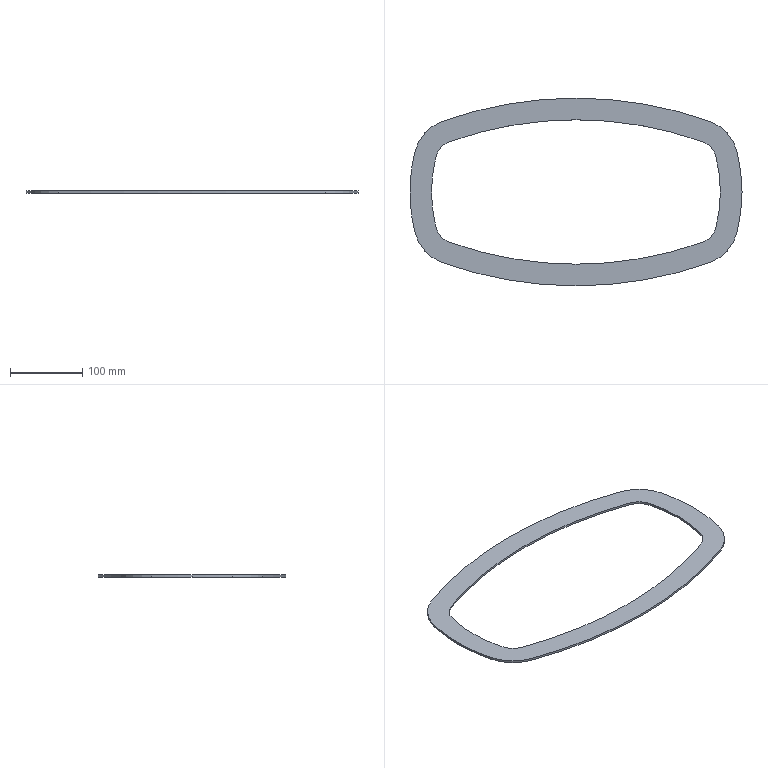Part | SolidWorks | features Extrusion 1 | 1 solid | 20 faces | box 460 x 260 x 3 mm | volume 101049 mm3 | cylinder 18 | plane 2 | commonest cylinder face diameters 60 x4 120 x4 400 x3 460 x3 1040 x2 1100 x2
STEP:
#1=CARTESIAN_POINT('',(-193.97,48.739,3.));
#2=VERTEX_POINT('',#1);
#3=CARTESIAN_POINT('',(-200.,0.,3.));
#4=VERTEX_POINT('',#3);
#5=CARTESIAN_POINT('',(0.,0.,3.));
#6=DIRECTION('',(0.,0.,1.));
#7=DIRECTION('',(-1.,0.,0.));
#8=AXIS2_PLACEMENT_3D('',#5,#6,#7);
#9=CIRCLE('',#8,200.);
#10=EDGE_CURVE('',#2,#4,#9,.T.);
#11=ORIENTED_EDGE('',*,*,#10,.T.);
#12=CARTESIAN_POINT('',(-200.,0.,0.));
#13=VERTEX_POINT('',#12);
#14=CARTESIAN_POINT('',(-200.,0.,3.));
#15=DIRECTION('',(0.,0.,-1.));
#16=VECTOR('',#15,1000.);
#17=LINE('',#14,#16);
#18=EDGE_CURVE('',#4,#13,#17,.T.);
#19=ORIENTED_EDGE('',*,*,#18,.T.);
#20=CARTESIAN_POINT('',(-193.97,48.739,0.));
#21=VERTEX_POINT('',#20);
#22=CARTESIAN_POINT('',(0.,0.,0.));
#23=DIRECTION('',(0.,0.,1.));
#24=DIRECTION('',(-1.,0.,0.));
#25=AXIS2_PLACEMENT_3D('',#22,#23,#24);
#26=CIRCLE('',#25,200.);
#27=EDGE_CURVE('',#21,#13,#26,.T.);
#28=ORIENTED_EDGE('',*,*,#27,.F.);
#29=CARTESIAN_POINT('',(-193.97,48.739,3.));
#30=DIRECTION('',(0.,0.,-1.));
#31=VECTOR('',#30,1000.);
#32=LINE('',#29,#31);
#33=EDGE_CURVE('',#2,#21,#32,.T.);
#34=ORIENTED_EDGE('',*,*,#33,.F.);
#35=EDGE_LOOP('',(#11,#19,#28,#34));
#36=FACE_OUTER_BOUND('',#35,.T.);
#37=CARTESIAN_POINT('',(0.,0.,3.));
#38=DIRECTION('',(0.,0.,-1.));
#39=DIRECTION('',(-1.,0.,0.));
#40=AXIS2_PLACEMENT_3D('',#37,#38,#39);
#41=CYLINDRICAL_SURFACE('',#40,200.);
#42=ADVANCED_FACE('',(#36),#41,.F.);
#43=CARTESIAN_POINT('',(-230.,0.,3.));
#44=VERTEX_POINT('',#43);
#45=CARTESIAN_POINT('',(-223.066,-56.05,3.));
#46=VERTEX_POINT('',#45);
#47=CARTESIAN_POINT('',(0.,0.,3.));
#48=DIRECTION('',(0.,0.,1.));
#49=DIRECTION('',(-1.,0.,0.));
#50=AXIS2_PLACEMENT_3D('',#47,#48,#49);
#51=CIRCLE('',#50,230.);
#52=EDGE_CURVE('',#44,#46,#51,.T.);
#53=ORIENTED_EDGE('',*,*,#52,.F.);
#54=CARTESIAN_POINT('',(-230.,0.,0.));
#55=VERTEX_POINT('',#54);
#56=CARTESIAN_POINT('',(-230.,0.,3.));
#57=DIRECTION('',(0.,0.,-1.));
#58=VECTOR('',#57,1000.);
#59=LINE('',#56,#58);
#60=EDGE_CURVE('',#44,#55,#59,.T.);
#61=ORIENTED_EDGE('',*,*,#60,.T.);
#62=CARTESIAN_POINT('',(-223.066,-56.05,0.));
#63=VERTEX_POINT('',#62);
#64=CARTESIAN_POINT('',(0.,0.,0.));
#65=DIRECTION('',(0.,0.,1.));
#66=DIRECTION('',(-1.,0.,0.));
#67=AXIS2_PLACEMENT_3D('',#64,#65,#66);
#68=CIRCLE('',#67,230.);
#69=EDGE_CURVE('',#55,#63,#68,.T.);
#70=ORIENTED_EDGE('',*,*,#69,.T.);
#71=CARTESIAN_POINT('',(-223.066,-56.05,3.));
#72=DIRECTION('',(0.,0.,-1.));
#73=VECTOR('',#72,1000.);
#74=LINE('',#71,#73);
#75=EDGE_CURVE('',#46,#63,#74,.T.);
#76=ORIENTED_EDGE('',*,*,#75,.F.);
#77=EDGE_LOOP('',(#53,#61,#70,#76));
#78=FACE_OUTER_BOUND('',#77,.T.);
#79=CARTESIAN_POINT('',(0.,0.,3.));
#80=DIRECTION('',(0.,0.,-1.));
#81=DIRECTION('',(-1.,0.,0.));
#82=AXIS2_PLACEMENT_3D('',#79,#80,#81);
#83=CYLINDRICAL_SURFACE('',#82,230.);
#84=ADVANCED_FACE('',(#78),#83,.T.);
#85=CARTESIAN_POINT('',(-185.063,97.93,3.));
#86=VERTEX_POINT('',#85);
#87=CARTESIAN_POINT('',(-223.066,56.05,3.));
#88=VERTEX_POINT('',#87);
#89=CARTESIAN_POINT('',(-164.875,41.429,3.));
#90=DIRECTION('',(0.,0.,1.));
#91=DIRECTION('',(1.,0.,0.));
#92=AXIS2_PLACEMENT_3D('',#89,#90,#91);
#93=CIRCLE('',#92,60.);
#94=EDGE_CURVE('',#86,#88,#93,.T.);
#95=ORIENTED_EDGE('',*,*,#94,.T.);
#96=CARTESIAN_POINT('',(0.,0.,3.));
#97=DIRECTION('',(0.,0.,1.));
#98=DIRECTION('',(-1.,0.,0.));
#99=AXIS2_PLACEMENT_3D('',#96,#97,#98);
#100=CIRCLE('',#99,230.);
#101=EDGE_CURVE('',#88,#44,#100,.T.);
#102=ORIENTED_EDGE('',*,*,#101,.T.);
#103=ORIENTED_EDGE('',*,*,#52,.T.);
#104=CARTESIAN_POINT('',(-185.063,-97.93,3.));
#105=VERTEX_POINT('',#104);
#106=CARTESIAN_POINT('',(-164.875,-41.429,3.));
#107=DIRECTION('',(0.,0.,1.));
#108=DIRECTION('',(-1.,0.,0.));
#109=AXIS2_PLACEMENT_3D('',#106,#107,#108);
#110=CIRCLE('',#109,60.);
#111=EDGE_CURVE('',#46,#105,#110,.T.);
#112=ORIENTED_EDGE('',*,*,#111,.T.);
#113=CARTESIAN_POINT('',(185.063,-97.93,3.));
#114=VERTEX_POINT('',#113);
#115=CARTESIAN_POINT('',(0.,420.,3.));
#116=DIRECTION('',(0.,0.,1.));
#117=DIRECTION('',(1.,0.,0.));
#118=AXIS2_PLACEMENT_3D('',#115,#116,#117);
#119=CIRCLE('',#118,550.);
#120=EDGE_CURVE('',#105,#114,#119,.T.);
#121=ORIENTED_EDGE('',*,*,#120,.T.);
#122=CARTESIAN_POINT('',(223.066,-56.05,3.));
#123=VERTEX_POINT('',#122);
#124=CARTESIAN_POINT('',(164.875,-41.429,3.));
#125=DIRECTION('',(0.,0.,1.));
#126=DIRECTION('',(1.,0.,0.));
#127=AXIS2_PLACEMENT_3D('',#124,#125,#126);
#128=CIRCLE('',#127,60.);
#129=EDGE_CURVE('',#114,#123,#128,.T.);
#130=ORIENTED_EDGE('',*,*,#129,.T.);
#131=CARTESIAN_POINT('',(223.066,56.05,3.));
#132=VERTEX_POINT('',#131);
#133=CARTESIAN_POINT('',(0.,0.,3.));
#134=DIRECTION('',(0.,0.,1.));
#135=DIRECTION('',(-1.,0.,0.));
#136=AXIS2_PLACEMENT_3D('',#133,#134,#135);
#137=CIRCLE('',#136,230.);
#138=EDGE_CURVE('',#123,#132,#137,.T.);
#139=ORIENTED_EDGE('',*,*,#138,.T.);
#140=CARTESIAN_POINT('',(185.063,97.93,3.));
#141=VERTEX_POINT('',#140);
#142=CARTESIAN_POINT('',(164.875,41.429,3.));
#143=DIRECTION('',(0.,0.,1.));
#144=DIRECTION('',(-1.,0.,0.));
#145=AXIS2_PLACEMENT_3D('',#142,#143,#144);
#146=CIRCLE('',#145,60.);
#147=EDGE_CURVE('',#132,#141,#146,.T.);
#148=ORIENTED_EDGE('',*,*,#147,.T.);
#149=CARTESIAN_POINT('',(0.,-420.,3.));
#150=DIRECTION('',(0.,0.,1.));
#151=DIRECTION('',(-1.,0.,0.));
#152=AXIS2_PLACEMENT_3D('',#149,#150,#151);
#153=CIRCLE('',#152,550.);
#154=EDGE_CURVE('',#141,#86,#153,.T.);
#155=ORIENTED_EDGE('',*,*,#154,.T.);
#156=EDGE_LOOP('',(#95,#102,#103,#112,#121,#130,#139,#148,#155));
#157=FACE_OUTER_BOUND('',#156,.T.);
#158=CARTESIAN_POINT('',(193.97,-48.739,3.));
#159=VERTEX_POINT('',#158);
#160=CARTESIAN_POINT('',(193.97,48.739,3.));
#161=VERTEX_POINT('',#160);
#162=CARTESIAN_POINT('',(0.,0.,3.));
#163=DIRECTION('',(0.,0.,1.));
#164=DIRECTION('',(-1.,0.,0.));
#165=AXIS2_PLACEMENT_3D('',#162,#163,#164);
#166=CIRCLE('',#165,200.);
#167=EDGE_CURVE('',#159,#161,#166,.T.);
#168=ORIENTED_EDGE('',*,*,#167,.F.);
#169=CARTESIAN_POINT('',(174.969,-69.679,3.));
#170=VERTEX_POINT('',#169);
#171=CARTESIAN_POINT('',(164.875,-41.429,3.));
#172=DIRECTION('',(0.,0.,1.));
#173=DIRECTION('',(1.,0.,0.));
#174=AXIS2_PLACEMENT_3D('',#171,#172,#173);
#175=CIRCLE('',#174,30.);
#176=EDGE_CURVE('',#170,#159,#175,.T.);
#177=ORIENTED_EDGE('',*,*,#176,.F.);
#178=CARTESIAN_POINT('',(-174.969,-69.679,3.));
#179=VERTEX_POINT('',#178);
#180=CARTESIAN_POINT('',(0.,420.,3.));
#181=DIRECTION('',(0.,0.,1.));
#182=DIRECTION('',(1.,0.,0.));
#183=AXIS2_PLACEMENT_3D('',#180,#181,#182);
#184=CIRCLE('',#183,520.);
#185=EDGE_CURVE('',#179,#170,#184,.T.);
#186=ORIENTED_EDGE('',*,*,#185,.F.);
#187=CARTESIAN_POINT('',(-193.97,-48.739,3.));
#188=VERTEX_POINT('',#187);
#189=CARTESIAN_POINT('',(-164.875,-41.429,3.));
#190=DIRECTION('',(0.,0.,1.));
#191=DIRECTION('',(-1.,0.,0.));
#192=AXIS2_PLACEMENT_3D('',#189,#190,#191);
#193=CIRCLE('',#192,30.);
#194=EDGE_CURVE('',#188,#179,#193,.T.);
#195=ORIENTED_EDGE('',*,*,#194,.F.);
#196=CARTESIAN_POINT('',(0.,0.,3.));
#197=DIRECTION('',(0.,0.,1.));
#198=DIRECTION('',(-1.,0.,0.));
#199=AXIS2_PLACEMENT_3D('',#196,#197,#198);
#200=CIRCLE('',#199,200.);
#201=EDGE_CURVE('',#4,#188,#200,.T.);
#202=ORIENTED_EDGE('',*,*,#201,.F.);
#203=ORIENTED_EDGE('',*,*,#10,.F.);
#204=CARTESIAN_POINT('',(-174.969,69.679,3.));
#205=VERTEX_POINT('',#204);
#206=CARTESIAN_POINT('',(-164.875,41.429,3.));
#207=DIRECTION('',(0.,0.,1.));
#208=DIRECTION('',(1.,0.,0.));
#209=AXIS2_PLACEMENT_3D('',#206,#207,#208);
#210=CIRCLE('',#209,30.);
#211=EDGE_CURVE('',#205,#2,#210,.T.);
#212=ORIENTED_EDGE('',*,*,#211,.F.);
#213=CARTESIAN_POINT('',(174.969,69.679,3.));
#214=VERTEX_POINT('',#213);
#215=CARTESIAN_POINT('',(0.,-420.,3.));
#216=DIRECTION('',(0.,0.,1.));
#217=DIRECTION('',(-1.,0.,0.));
#218=AXIS2_PLACEMENT_3D('',#215,#216,#217);
#219=CIRCLE('',#218,520.);
#220=EDGE_CURVE('',#214,#205,#219,.T.);
#221=ORIENTED_EDGE('',*,*,#220,.F.);
#222=CARTESIAN_POINT('',(164.875,41.429,3.));
#223=DIRECTION('',(0.,0.,1.));
#224=DIRECTION('',(-1.,0.,0.));
#225=AXIS2_PLACEMENT_3D('',#222,#223,#224);
#226=CIRCLE('',#225,30.);
#227=EDGE_CURVE('',#161,#214,#226,.T.);
#228=ORIENTED_EDGE('',*,*,#227,.F.);
#229=EDGE_LOOP('',(#168,#177,#186,#195,#202,#203,#212,#221,#228));
#230=FACE_BOUND('',#229,.T.);
#231=CARTESIAN_POINT('',(-82.437,20.714,3.));
#232=DIRECTION('',(0.,0.,1.));
#233=DIRECTION('',(1.,0.,0.));
#234=AXIS2_PLACEMENT_3D('',#231,#232,#233);
#235=PLANE('',#234);
#236=ADVANCED_FACE('',(#157,#230),#235,.T.);
#237=CARTESIAN_POINT('',(-185.063,97.93,0.));
#238=VERTEX_POINT('',#237);
#239=CARTESIAN_POINT('',(-223.066,56.05,0.));
#240=VERTEX_POINT('',#239);
#241=CARTESIAN_POINT('',(-164.875,41.429,0.));
#242=DIRECTION('',(0.,0.,1.));
#243=DIRECTION('',(1.,0.,0.));
#244=AXIS2_PLACEMENT_3D('',#241,#242,#243);
#245=CIRCLE('',#244,60.);
#246=EDGE_CURVE('',#238,#240,#245,.T.);
#247=ORIENTED_EDGE('',*,*,#246,.F.);
#248=CARTESIAN_POINT('',(185.063,97.93,0.));
#249=VERTEX_POINT('',#248);
#250=CARTESIAN_POINT('',(0.,-420.,0.));
#251=DIRECTION('',(0.,0.,1.));
#252=DIRECTION('',(-1.,0.,0.));
#253=AXIS2_PLACEMENT_3D('',#250,#251,#252);
#254=CIRCLE('',#253,550.);
#255=EDGE_CURVE('',#249,#238,#254,.T.);
#256=ORIENTED_EDGE('',*,*,#255,.F.);
#257=CARTESIAN_POINT('',(223.066,56.05,0.));
#258=VERTEX_POINT('',#257);
#259=CARTESIAN_POINT('',(164.875,41.429,0.));
#260=DIRECTION('',(0.,0.,1.));
#261=DIRECTION('',(-1.,0.,0.));
#262=AXIS2_PLACEMENT_3D('',#259,#260,#261);
#263=CIRCLE('',#262,60.);
#264=EDGE_CURVE('',#258,#249,#263,.T.);
#265=ORIENTED_EDGE('',*,*,#264,.F.);
#266=CARTESIAN_POINT('',(223.066,-56.05,0.));
#267=VERTEX_POINT('',#266);
#268=CARTESIAN_POINT('',(0.,0.,0.));
#269=DIRECTION('',(0.,0.,1.));
#270=DIRECTION('',(-1.,0.,0.));
#271=AXIS2_PLACEMENT_3D('',#268,#269,#270);
#272=CIRCLE('',#271,230.);
#273=EDGE_CURVE('',#267,#258,#272,.T.);
#274=ORIENTED_EDGE('',*,*,#273,.F.);
#275=CARTESIAN_POINT('',(185.063,-97.93,0.));
#276=VERTEX_POINT('',#275);
#277=CARTESIAN_POINT('',(164.875,-41.429,0.));
#278=DIRECTION('',(0.,0.,1.));
#279=DIRECTION('',(1.,0.,0.));
#280=AXIS2_PLACEMENT_3D('',#277,#278,#279);
#281=CIRCLE('',#280,60.);
#282=EDGE_CURVE('',#276,#267,#281,.T.);
#283=ORIENTED_EDGE('',*,*,#282,.F.);
#284=CARTESIAN_POINT('',(-185.063,-97.93,0.));
#285=VERTEX_POINT('',#284);
#286=CARTESIAN_POINT('',(0.,420.,0.));
#287=DIRECTION('',(0.,0.,1.));
#288=DIRECTION('',(1.,0.,0.));
#289=AXIS2_PLACEMENT_3D('',#286,#287,#288);
#290=CIRCLE('',#289,550.);
#291=EDGE_CURVE('',#285,#276,#290,.T.);
#292=ORIENTED_EDGE('',*,*,#291,.F.);
#293=CARTESIAN_POINT('',(-164.875,-41.429,0.));
#294=DIRECTION('',(0.,0.,1.));
#295=DIRECTION('',(-1.,0.,0.));
#296=AXIS2_PLACEMENT_3D('',#293,#294,#295);
#297=CIRCLE('',#296,60.);
#298=EDGE_CURVE('',#63,#285,#297,.T.);
#299=ORIENTED_EDGE('',*,*,#298,.F.);
#300=ORIENTED_EDGE('',*,*,#69,.F.);
#301=CARTESIAN_POINT('',(0.,0.,0.));
#302=DIRECTION('',(0.,0.,1.));
#303=DIRECTION('',(-1.,0.,0.));
#304=AXIS2_PLACEMENT_3D('',#301,#302,#303);
#305=CIRCLE('',#304,230.);
#306=EDGE_CURVE('',#240,#55,#305,.T.);
#307=ORIENTED_EDGE('',*,*,#306,.F.);
#308=EDGE_LOOP('',(#247,#256,#265,#274,#283,#292,#299,#300,#307));
#309=FACE_OUTER_BOUND('',#308,.T.);
#310=CARTESIAN_POINT('',(174.969,-69.679,0.));
#311=VERTEX_POINT('',#310);
#312=CARTESIAN_POINT('',(193.97,-48.739,0.));
#313=VERTEX_POINT('',#312);
#314=CARTESIAN_POINT('',(164.875,-41.429,0.));
#315=DIRECTION('',(0.,0.,1.));
#316=DIRECTION('',(1.,0.,0.));
#317=AXIS2_PLACEMENT_3D('',#314,#315,#316);
#318=CIRCLE('',#317,30.);
#319=EDGE_CURVE('',#311,#313,#318,.T.);
#320=ORIENTED_EDGE('',*,*,#319,.T.);
#321=CARTESIAN_POINT('',(193.97,48.739,0.));
#322=VERTEX_POINT('',#321);
#323=CARTESIAN_POINT('',(0.,0.,0.));
#324=DIRECTION('',(0.,0.,1.));
#325=DIRECTION('',(-1.,0.,0.));
#326=AXIS2_PLACEMENT_3D('',#323,#324,#325);
#327=CIRCLE('',#326,200.);
#328=EDGE_CURVE('',#313,#322,#327,.T.);
#329=ORIENTED_EDGE('',*,*,#328,.T.);
#330=CARTESIAN_POINT('',(174.969,69.679,0.));
#331=VERTEX_POINT('',#330);
#332=CARTESIAN_POINT('',(164.875,41.429,0.));
#333=DIRECTION('',(0.,0.,1.));
#334=DIRECTION('',(-1.,0.,0.));
#335=AXIS2_PLACEMENT_3D('',#332,#333,#334);
#336=CIRCLE('',#335,30.);
#337=EDGE_CURVE('',#322,#331,#336,.T.);
#338=ORIENTED_EDGE('',*,*,#337,.T.);
#339=CARTESIAN_POINT('',(-174.969,69.679,0.));
#340=VERTEX_POINT('',#339);
#341=CARTESIAN_POINT('',(0.,-420.,0.));
#342=DIRECTION('',(0.,0.,1.));
#343=DIRECTION('',(-1.,0.,0.));
#344=AXIS2_PLACEMENT_3D('',#341,#342,#343);
#345=CIRCLE('',#344,520.);
#346=EDGE_CURVE('',#331,#340,#345,.T.);
#347=ORIENTED_EDGE('',*,*,#346,.T.);
#348=CARTESIAN_POINT('',(-164.875,41.429,0.));
#349=DIRECTION('',(0.,0.,1.));
#350=DIRECTION('',(1.,0.,0.));
#351=AXIS2_PLACEMENT_3D('',#348,#349,#350);
#352=CIRCLE('',#351,30.);
#353=EDGE_CURVE('',#340,#21,#352,.T.);
#354=ORIENTED_EDGE('',*,*,#353,.T.);
#355=ORIENTED_EDGE('',*,*,#27,.T.);
#356=CARTESIAN_POINT('',(-193.97,-48.739,0.));
#357=VERTEX_POINT('',#356);
#358=CARTESIAN_POINT('',(0.,0.,0.));
#359=DIRECTION('',(0.,0.,1.));
#360=DIRECTION('',(-1.,0.,0.));
#361=AXIS2_PLACEMENT_3D('',#358,#359,#360);
#362=CIRCLE('',#361,200.);
#363=EDGE_CURVE('',#13,#357,#362,.T.);
#364=ORIENTED_EDGE('',*,*,#363,.T.);
#365=CARTESIAN_POINT('',(-174.969,-69.679,0.));
#366=VERTEX_POINT('',#365);
#367=CARTESIAN_POINT('',(-164.875,-41.429,0.));
#368=DIRECTION('',(0.,0.,1.));
#369=DIRECTION('',(-1.,0.,0.));
#370=AXIS2_PLACEMENT_3D('',#367,#368,#369);
#371=CIRCLE('',#370,30.);
#372=EDGE_CURVE('',#357,#366,#371,.T.);
#373=ORIENTED_EDGE('',*,*,#372,.T.);
#374=CARTESIAN_POINT('',(0.,420.,0.));
#375=DIRECTION('',(0.,0.,1.));
#376=DIRECTION('',(1.,0.,0.));
#377=AXIS2_PLACEMENT_3D('',#374,#375,#376);
#378=CIRCLE('',#377,520.);
#379=EDGE_CURVE('',#366,#311,#378,.T.);
#380=ORIENTED_EDGE('',*,*,#379,.T.);
#381=EDGE_LOOP('',(#320,#329,#338,#347,#354,#355,#364,#373,#380));
#382=FACE_BOUND('',#381,.T.);
#383=CARTESIAN_POINT('',(-82.437,20.714,0.));
#384=DIRECTION('',(0.,0.,1.));
#385=DIRECTION('',(1.,0.,0.));
#386=AXIS2_PLACEMENT_3D('',#383,#384,#385);
#387=PLANE('',#386);
#388=ADVANCED_FACE('',(#309,#382),#387,.F.);
#389=ORIENTED_EDGE('',*,*,#246,.T.);
#390=CARTESIAN_POINT('',(-223.066,56.05,3.));
#391=DIRECTION('',(0.,0.,-1.));
#392=VECTOR('',#391,1000.);
#393=LINE('',#390,#392);
#394=EDGE_CURVE('',#88,#240,#393,.T.);
#395=ORIENTED_EDGE('',*,*,#394,.F.);
#396=ORIENTED_EDGE('',*,*,#94,.F.);
#397=CARTESIAN_POINT('',(-185.063,97.93,3.));
#398=DIRECTION('',(0.,0.,-1.));
#399=VECTOR('',#398,1000.);
#400=LINE('',#397,#399);
#401=EDGE_CURVE('',#86,#238,#400,.T.);
#402=ORIENTED_EDGE('',*,*,#401,.T.);
#403=EDGE_LOOP('',(#389,#395,#396,#402));
#404=FACE_OUTER_BOUND('',#403,.T.);
#405=CARTESIAN_POINT('',(-164.875,41.429,3.));
#406=DIRECTION('',(0.,0.,-1.));
#407=DIRECTION('',(-1.,0.,0.));
#408=AXIS2_PLACEMENT_3D('',#405,#406,#407);
#409=CYLINDRICAL_SURFACE('',#408,60.);
#410=ADVANCED_FACE('',(#404),#409,.T.);
#411=ORIENTED_EDGE('',*,*,#60,.F.);
#412=ORIENTED_EDGE('',*,*,#101,.F.);
#413=ORIENTED_EDGE('',*,*,#394,.T.);
#414=ORIENTED_EDGE('',*,*,#306,.T.);
#415=EDGE_LOOP('',(#411,#412,#413,#414));
#416=FACE_OUTER_BOUND('',#415,.T.);
#417=CARTESIAN_POINT('',(0.,0.,3.));
#418=DIRECTION('',(0.,0.,-1.));
#419=DIRECTION('',(-1.,0.,0.));
#420=AXIS2_PLACEMENT_3D('',#417,#418,#419);
#421=CYLINDRICAL_SURFACE('',#420,230.);
#422=ADVANCED_FACE('',(#416),#421,.T.);
#423=ORIENTED_EDGE('',*,*,#298,.T.);
#424=CARTESIAN_POINT('',(-185.063,-97.93,3.));
#425=DIRECTION('',(0.,0.,-1.));
#426=VECTOR('',#425,1000.);
#427=LINE('',#424,#426);
#428=EDGE_CURVE('',#105,#285,#427,.T.);
#429=ORIENTED_EDGE('',*,*,#428,.F.);
#430=ORIENTED_EDGE('',*,*,#111,.F.);
#431=ORIENTED_EDGE('',*,*,#75,.T.);
#432=EDGE_LOOP('',(#423,#429,#430,#431));
#433=FACE_OUTER_BOUND('',#432,.T.);
#434=CARTESIAN_POINT('',(-164.875,-41.429,3.));
#435=DIRECTION('',(0.,0.,-1.));
#436=DIRECTION('',(-1.,0.,0.));
#437=AXIS2_PLACEMENT_3D('',#434,#435,#436);
#438=CYLINDRICAL_SURFACE('',#437,60.);
#439=ADVANCED_FACE('',(#433),#438,.T.);
#440=ORIENTED_EDGE('',*,*,#291,.T.);
#441=CARTESIAN_POINT('',(185.063,-97.93,3.));
#442=DIRECTION('',(0.,0.,-1.));
#443=VECTOR('',#442,1000.);
#444=LINE('',#441,#443);
#445=EDGE_CURVE('',#114,#276,#444,.T.);
#446=ORIENTED_EDGE('',*,*,#445,.F.);
#447=ORIENTED_EDGE('',*,*,#120,.F.);
#448=ORIENTED_EDGE('',*,*,#428,.T.);
#449=EDGE_LOOP('',(#440,#446,#447,#448));
#450=FACE_OUTER_BOUND('',#449,.T.);
#451=CARTESIAN_POINT('',(0.,420.,3.));
#452=DIRECTION('',(0.,0.,-1.));
#453=DIRECTION('',(-1.,0.,0.));
#454=AXIS2_PLACEMENT_3D('',#451,#452,#453);
#455=CYLINDRICAL_SURFACE('',#454,550.);
#456=ADVANCED_FACE('',(#450),#455,.T.);
#457=ORIENTED_EDGE('',*,*,#282,.T.);
#458=CARTESIAN_POINT('',(223.066,-56.05,3.));
#459=DIRECTION('',(0.,0.,-1.));
#460=VECTOR('',#459,1000.);
#461=LINE('',#458,#460);
#462=EDGE_CURVE('',#123,#267,#461,.T.);
#463=ORIENTED_EDGE('',*,*,#462,.F.);
#464=ORIENTED_EDGE('',*,*,#129,.F.);
#465=ORIENTED_EDGE('',*,*,#445,.T.);
#466=EDGE_LOOP('',(#457,#463,#464,#465));
#467=FACE_OUTER_BOUND('',#466,.T.);
#468=CARTESIAN_POINT('',(164.875,-41.429,3.));
#469=DIRECTION('',(0.,0.,-1.));
#470=DIRECTION('',(-1.,0.,0.));
#471=AXIS2_PLACEMENT_3D('',#468,#469,#470);
#472=CYLINDRICAL_SURFACE('',#471,60.);
#473=ADVANCED_FACE('',(#467),#472,.T.);
#474=ORIENTED_EDGE('',*,*,#273,.T.);
#475=CARTESIAN_POINT('',(223.066,56.05,3.));
#476=DIRECTION('',(0.,0.,-1.));
#477=VECTOR('',#476,1000.);
#478=LINE('',#475,#477);
#479=EDGE_CURVE('',#132,#258,#478,.T.);
#480=ORIENTED_EDGE('',*,*,#479,.F.);
#481=ORIENTED_EDGE('',*,*,#138,.F.);
#482=ORIENTED_EDGE('',*,*,#462,.T.);
#483=EDGE_LOOP('',(#474,#480,#481,#482));
#484=FACE_OUTER_BOUND('',#483,.T.);
#485=CARTESIAN_POINT('',(0.,0.,3.));
#486=DIRECTION('',(0.,0.,-1.));
#487=DIRECTION('',(-1.,0.,0.));
#488=AXIS2_PLACEMENT_3D('',#485,#486,#487);
#489=CYLINDRICAL_SURFACE('',#488,230.);
#490=ADVANCED_FACE('',(#484),#489,.T.);
#491=ORIENTED_EDGE('',*,*,#264,.T.);
#492=CARTESIAN_POINT('',(185.063,97.93,3.));
#493=DIRECTION('',(0.,0.,-1.));
#494=VECTOR('',#493,1000.);
#495=LINE('',#492,#494);
#496=EDGE_CURVE('',#141,#249,#495,.T.);
#497=ORIENTED_EDGE('',*,*,#496,.F.);
#498=ORIENTED_EDGE('',*,*,#147,.F.);
#499=ORIENTED_EDGE('',*,*,#479,.T.);
#500=EDGE_LOOP('',(#491,#497,#498,#499));
#501=FACE_OUTER_BOUND('',#500,.T.);
#502=CARTESIAN_POINT('',(164.875,41.429,3.));
#503=DIRECTION('',(0.,0.,-1.));
#504=DIRECTION('',(-1.,0.,0.));
#505=AXIS2_PLACEMENT_3D('',#502,#503,#504);
#506=CYLINDRICAL_SURFACE('',#505,60.);
#507=ADVANCED_FACE('',(#501),#506,.T.);
#508=ORIENTED_EDGE('',*,*,#255,.T.);
#509=ORIENTED_EDGE('',*,*,#401,.F.);
#510=ORIENTED_EDGE('',*,*,#154,.F.);
#511=ORIENTED_EDGE('',*,*,#496,.T.);
#512=EDGE_LOOP('',(#508,#509,#510,#511));
#513=FACE_OUTER_BOUND('',#512,.T.);
#514=CARTESIAN_POINT('',(0.,-420.,3.));
#515=DIRECTION('',(0.,0.,-1.));
#516=DIRECTION('',(-1.,0.,0.));
#517=AXIS2_PLACEMENT_3D('',#514,#515,#516);
#518=CYLINDRICAL_SURFACE('',#517,550.);
#519=ADVANCED_FACE('',(#513),#518,.T.);
#520=ORIENTED_EDGE('',*,*,#319,.F.);
#521=CARTESIAN_POINT('',(174.969,-69.679,3.));
#522=DIRECTION('',(0.,0.,-1.));
#523=VECTOR('',#522,1000.);
#524=LINE('',#521,#523);
#525=EDGE_CURVE('',#170,#311,#524,.T.);
#526=ORIENTED_EDGE('',*,*,#525,.F.);
#527=ORIENTED_EDGE('',*,*,#176,.T.);
#528=CARTESIAN_POINT('',(193.97,-48.739,3.));
#529=DIRECTION('',(0.,0.,-1.));
#530=VECTOR('',#529,1000.);
#531=LINE('',#528,#530);
#532=EDGE_CURVE('',#159,#313,#531,.T.);
#533=ORIENTED_EDGE('',*,*,#532,.T.);
#534=EDGE_LOOP('',(#520,#526,#527,#533));
#535=FACE_OUTER_BOUND('',#534,.T.);
#536=CARTESIAN_POINT('',(164.875,-41.429,3.));
#537=DIRECTION('',(0.,0.,-1.));
#538=DIRECTION('',(-1.,0.,0.));
#539=AXIS2_PLACEMENT_3D('',#536,#537,#538);
#540=CYLINDRICAL_SURFACE('',#539,30.);
#541=ADVANCED_FACE('',(#535),#540,.F.);
#542=ORIENTED_EDGE('',*,*,#328,.F.);
#543=ORIENTED_EDGE('',*,*,#532,.F.);
#544=ORIENTED_EDGE('',*,*,#167,.T.);
#545=CARTESIAN_POINT('',(193.97,48.739,3.));
#546=DIRECTION('',(0.,0.,-1.));
#547=VECTOR('',#546,1000.);
#548=LINE('',#545,#547);
#549=EDGE_CURVE('',#161,#322,#548,.T.);
#550=ORIENTED_EDGE('',*,*,#549,.T.);
#551=EDGE_LOOP('',(#542,#543,#544,#550));
#552=FACE_OUTER_BOUND('',#551,.T.);
#553=CARTESIAN_POINT('',(0.,0.,3.));
#554=DIRECTION('',(0.,0.,-1.));
#555=DIRECTION('',(-1.,0.,0.));
#556=AXIS2_PLACEMENT_3D('',#553,#554,#555);
#557=CYLINDRICAL_SURFACE('',#556,200.);
#558=ADVANCED_FACE('',(#552),#557,.F.);
#559=ORIENTED_EDGE('',*,*,#337,.F.);
#560=ORIENTED_EDGE('',*,*,#549,.F.);
#561=ORIENTED_EDGE('',*,*,#227,.T.);
#562=CARTESIAN_POINT('',(174.969,69.679,3.));
#563=DIRECTION('',(0.,0.,-1.));
#564=VECTOR('',#563,1000.);
#565=LINE('',#562,#564);
#566=EDGE_CURVE('',#214,#331,#565,.T.);
#567=ORIENTED_EDGE('',*,*,#566,.T.);
#568=EDGE_LOOP('',(#559,#560,#561,#567));
#569=FACE_OUTER_BOUND('',#568,.T.);
#570=CARTESIAN_POINT('',(164.875,41.429,3.));
#571=DIRECTION('',(0.,0.,-1.));
#572=DIRECTION('',(-1.,0.,0.));
#573=AXIS2_PLACEMENT_3D('',#570,#571,#572);
#574=CYLINDRICAL_SURFACE('',#573,30.);
#575=ADVANCED_FACE('',(#569),#574,.F.);
#576=ORIENTED_EDGE('',*,*,#346,.F.);
#577=ORIENTED_EDGE('',*,*,#566,.F.);
#578=ORIENTED_EDGE('',*,*,#220,.T.);
#579=CARTESIAN_POINT('',(-174.969,69.679,3.));
#580=DIRECTION('',(0.,0.,-1.));
#581=VECTOR('',#580,1000.);
#582=LINE('',#579,#581);
#583=EDGE_CURVE('',#205,#340,#582,.T.);
#584=ORIENTED_EDGE('',*,*,#583,.T.);
#585=EDGE_LOOP('',(#576,#577,#578,#584));
#586=FACE_OUTER_BOUND('',#585,.T.);
#587=CARTESIAN_POINT('',(0.,-420.,3.));
#588=DIRECTION('',(0.,0.,-1.));
#589=DIRECTION('',(-1.,0.,0.));
#590=AXIS2_PLACEMENT_3D('',#587,#588,#589);
#591=CYLINDRICAL_SURFACE('',#590,520.);
#592=ADVANCED_FACE('',(#586),#591,.F.);
#593=ORIENTED_EDGE('',*,*,#353,.F.);
#594=ORIENTED_EDGE('',*,*,#583,.F.);
#595=ORIENTED_EDGE('',*,*,#211,.T.);
#596=ORIENTED_EDGE('',*,*,#33,.T.);
#597=EDGE_LOOP('',(#593,#594,#595,#596));
#598=FACE_OUTER_BOUND('',#597,.T.);
#599=CARTESIAN_POINT('',(-164.875,41.429,3.));
#600=DIRECTION('',(0.,0.,-1.));
#601=DIRECTION('',(-1.,0.,0.));
#602=AXIS2_PLACEMENT_3D('',#599,#600,#601);
#603=CYLINDRICAL_SURFACE('',#602,30.);
#604=ADVANCED_FACE('',(#598),#603,.F.);
#605=ORIENTED_EDGE('',*,*,#18,.F.);
#606=ORIENTED_EDGE('',*,*,#201,.T.);
#607=CARTESIAN_POINT('',(-193.97,-48.739,3.));
#608=DIRECTION('',(0.,0.,-1.));
#609=VECTOR('',#608,1000.);
#610=LINE('',#607,#609);
#611=EDGE_CURVE('',#188,#357,#610,.T.);
#612=ORIENTED_EDGE('',*,*,#611,.T.);
#613=ORIENTED_EDGE('',*,*,#363,.F.);
#614=EDGE_LOOP('',(#605,#606,#612,#613));
#615=FACE_OUTER_BOUND('',#614,.T.);
#616=CARTESIAN_POINT('',(0.,0.,3.));
#617=DIRECTION('',(0.,0.,-1.));
#618=DIRECTION('',(-1.,0.,0.));
#619=AXIS2_PLACEMENT_3D('',#616,#617,#618);
#620=CYLINDRICAL_SURFACE('',#619,200.);
#621=ADVANCED_FACE('',(#615),#620,.F.);
#622=ORIENTED_EDGE('',*,*,#372,.F.);
#623=ORIENTED_EDGE('',*,*,#611,.F.);
#624=ORIENTED_EDGE('',*,*,#194,.T.);
#625=CARTESIAN_POINT('',(-174.969,-69.679,3.));
#626=DIRECTION('',(0.,0.,-1.));
#627=VECTOR('',#626,1000.);
#628=LINE('',#625,#627);
#629=EDGE_CURVE('',#179,#366,#628,.T.);
#630=ORIENTED_EDGE('',*,*,#629,.T.);
#631=EDGE_LOOP('',(#622,#623,#624,#630));
#632=FACE_OUTER_BOUND('',#631,.T.);
#633=CARTESIAN_POINT('',(-164.875,-41.429,3.));
#634=DIRECTION('',(0.,0.,-1.));
#635=DIRECTION('',(-1.,0.,0.));
#636=AXIS2_PLACEMENT_3D('',#633,#634,#635);
#637=CYLINDRICAL_SURFACE('',#636,30.);
#638=ADVANCED_FACE('',(#632),#637,.F.);
#639=ORIENTED_EDGE('',*,*,#379,.F.);
#640=ORIENTED_EDGE('',*,*,#629,.F.);
#641=ORIENTED_EDGE('',*,*,#185,.T.);
#642=ORIENTED_EDGE('',*,*,#525,.T.);
#643=EDGE_LOOP('',(#639,#640,#641,#642));
#644=FACE_OUTER_BOUND('',#643,.T.);
#645=CARTESIAN_POINT('',(0.,420.,3.));
#646=DIRECTION('',(0.,0.,-1.));
#647=DIRECTION('',(-1.,0.,0.));
#648=AXIS2_PLACEMENT_3D('',#645,#646,#647);
#649=CYLINDRICAL_SURFACE('',#648,520.);
#650=ADVANCED_FACE('',(#644),#649,.F.);
#651=CLOSED_SHELL('',(#42,#84,#236,#388,#410,#422,#439,#456,#473,#490,#507,#519,#541,#558,#575,#592,#604,#621,#638,#650));
#652=MANIFOLD_SOLID_BREP('',#651);
#653=CARTESIAN_POINT('',(0.,0.,0.));
#654=DIRECTION('',(0.,0.,1.));
#655=DIRECTION('',(1.,0.,0.));
#656=AXIS2_PLACEMENT_3D('',#653,#654,#655);
#657=(LENGTH_UNIT()NAMED_UNIT(*)SI_UNIT(.MILLI.,.METRE.));
#658=UNCERTAINTY_MEASURE_WITH_UNIT(LENGTH_MEASURE(0.00001),#657,'','');
#659=(NAMED_UNIT(*)PLANE_ANGLE_UNIT()SI_UNIT($,.RADIAN.));
#660=(NAMED_UNIT(*)SI_UNIT($,.STERADIAN.)SOLID_ANGLE_UNIT());
#661=(GEOMETRIC_REPRESENTATION_CONTEXT(3)GLOBAL_UNCERTAINTY_ASSIGNED_CONTEXT((#658))GLOBAL_UNIT_ASSIGNED_CONTEXT((#657,#659,#660))REPRESENTATION_CONTEXT('',''));
#662=ADVANCED_BREP_SHAPE_REPRESENTATION('',(#652,#656),#661);